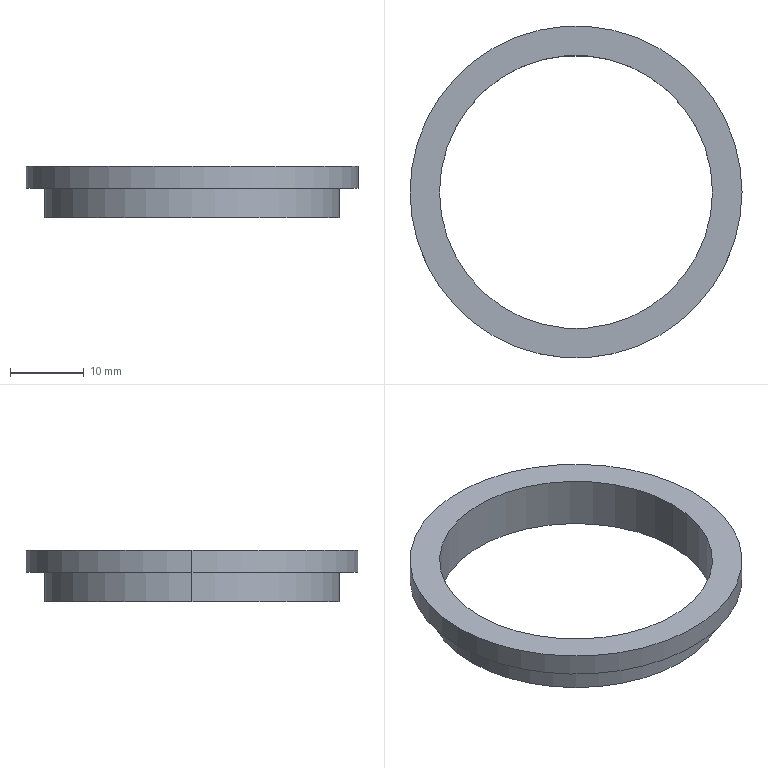Part | SolidWorks | features Extrusion 1, ICE 1 | 1 solid | 9 faces | box 45 x 45 x 7 mm | volume 2271 mm3 | cylinder 6 | plane 3 | commonest cylinder face diameters 37 x2 40 x2 45 x2
STEP:
#1=CARTESIAN_POINT('',(-20.,0.,-4.));
#2=VERTEX_POINT('',#1);
#3=CARTESIAN_POINT('',(20.,0.,-4.));
#4=VERTEX_POINT('',#3);
#5=CARTESIAN_POINT('',(0.,0.,-4.));
#6=DIRECTION('',(0.,0.,-1.));
#7=DIRECTION('',(-1.,0.,0.));
#8=AXIS2_PLACEMENT_3D('',#5,#6,#7);
#9=CIRCLE('',#8,20.);
#10=EDGE_CURVE('',#2,#4,#9,.T.);
#11=ORIENTED_EDGE('',*,*,#10,.F.);
#12=CARTESIAN_POINT('',(-20.,0.,0.));
#13=VERTEX_POINT('',#12);
#14=CARTESIAN_POINT('',(-20.,0.,-4.));
#15=DIRECTION('',(0.,0.,1.));
#16=VECTOR('',#15,1000.);
#17=LINE('',#14,#16);
#18=EDGE_CURVE('',#2,#13,#17,.T.);
#19=ORIENTED_EDGE('',*,*,#18,.T.);
#20=CARTESIAN_POINT('',(20.,0.,0.));
#21=VERTEX_POINT('',#20);
#22=CARTESIAN_POINT('',(0.,0.,0.));
#23=DIRECTION('',(0.,0.,-1.));
#24=DIRECTION('',(1.,0.,0.));
#25=AXIS2_PLACEMENT_3D('',#22,#23,#24);
#26=CIRCLE('',#25,20.);
#27=EDGE_CURVE('',#13,#21,#26,.T.);
#28=ORIENTED_EDGE('',*,*,#27,.T.);
#29=CARTESIAN_POINT('',(20.,0.,-4.));
#30=DIRECTION('',(0.,0.,1.));
#31=VECTOR('',#30,1000.);
#32=LINE('',#29,#31);
#33=EDGE_CURVE('',#4,#21,#32,.T.);
#34=ORIENTED_EDGE('',*,*,#33,.F.);
#35=EDGE_LOOP('',(#11,#19,#28,#34));
#36=FACE_OUTER_BOUND('',#35,.T.);
#37=CARTESIAN_POINT('',(0.,0.,-4.));
#38=DIRECTION('',(0.,0.,1.));
#39=DIRECTION('',(1.,0.,0.));
#40=AXIS2_PLACEMENT_3D('',#37,#38,#39);
#41=CYLINDRICAL_SURFACE('',#40,20.);
#42=ADVANCED_FACE('',(#36),#41,.T.);
#43=CARTESIAN_POINT('',(-18.5,0.,3.));
#44=VERTEX_POINT('',#43);
#45=CARTESIAN_POINT('',(18.5,0.,3.));
#46=VERTEX_POINT('',#45);
#47=CARTESIAN_POINT('',(0.,0.,3.));
#48=DIRECTION('',(0.,0.,1.));
#49=DIRECTION('',(1.,0.,0.));
#50=AXIS2_PLACEMENT_3D('',#47,#48,#49);
#51=CIRCLE('',#50,18.5);
#52=EDGE_CURVE('',#44,#46,#51,.T.);
#53=ORIENTED_EDGE('',*,*,#52,.T.);
#54=CARTESIAN_POINT('',(18.5,0.,-4.));
#55=VERTEX_POINT('',#54);
#56=CARTESIAN_POINT('',(18.5,0.,3.));
#57=DIRECTION('',(0.,0.,-1.));
#58=VECTOR('',#57,1000.);
#59=LINE('',#56,#58);
#60=EDGE_CURVE('',#46,#55,#59,.T.);
#61=ORIENTED_EDGE('',*,*,#60,.T.);
#62=CARTESIAN_POINT('',(-18.5,0.,-4.));
#63=VERTEX_POINT('',#62);
#64=CARTESIAN_POINT('',(0.,0.,-4.));
#65=DIRECTION('',(0.,0.,-1.));
#66=DIRECTION('',(-1.,0.,0.));
#67=AXIS2_PLACEMENT_3D('',#64,#65,#66);
#68=CIRCLE('',#67,18.5);
#69=EDGE_CURVE('',#55,#63,#68,.T.);
#70=ORIENTED_EDGE('',*,*,#69,.T.);
#71=CARTESIAN_POINT('',(-18.5,0.,3.));
#72=DIRECTION('',(0.,0.,-1.));
#73=VECTOR('',#72,1000.);
#74=LINE('',#71,#73);
#75=EDGE_CURVE('',#44,#63,#74,.T.);
#76=ORIENTED_EDGE('',*,*,#75,.F.);
#77=EDGE_LOOP('',(#53,#61,#70,#76));
#78=FACE_OUTER_BOUND('',#77,.T.);
#79=CARTESIAN_POINT('',(0.,0.,3.));
#80=DIRECTION('',(0.,0.,-1.));
#81=DIRECTION('',(-1.,0.,0.));
#82=AXIS2_PLACEMENT_3D('',#79,#80,#81);
#83=CYLINDRICAL_SURFACE('',#82,18.5);
#84=ADVANCED_FACE('',(#78),#83,.F.);
#85=CARTESIAN_POINT('',(22.5,0.,3.));
#86=VERTEX_POINT('',#85);
#87=CARTESIAN_POINT('',(-22.5,0.,3.));
#88=VERTEX_POINT('',#87);
#89=CARTESIAN_POINT('',(0.,0.,3.));
#90=DIRECTION('',(0.,0.,1.));
#91=DIRECTION('',(1.,0.,0.));
#92=AXIS2_PLACEMENT_3D('',#89,#90,#91);
#93=CIRCLE('',#92,22.5);
#94=EDGE_CURVE('',#86,#88,#93,.T.);
#95=ORIENTED_EDGE('',*,*,#94,.F.);
#96=CARTESIAN_POINT('',(22.5,0.,0.));
#97=VERTEX_POINT('',#96);
#98=CARTESIAN_POINT('',(22.5,0.,3.));
#99=DIRECTION('',(0.,0.,-1.));
#100=VECTOR('',#99,1000.);
#101=LINE('',#98,#100);
#102=EDGE_CURVE('',#86,#97,#101,.T.);
#103=ORIENTED_EDGE('',*,*,#102,.T.);
#104=CARTESIAN_POINT('',(-22.5,0.,0.));
#105=VERTEX_POINT('',#104);
#106=CARTESIAN_POINT('',(0.,0.,0.));
#107=DIRECTION('',(0.,0.,1.));
#108=DIRECTION('',(1.,0.,0.));
#109=AXIS2_PLACEMENT_3D('',#106,#107,#108);
#110=CIRCLE('',#109,22.5);
#111=EDGE_CURVE('',#97,#105,#110,.T.);
#112=ORIENTED_EDGE('',*,*,#111,.T.);
#113=CARTESIAN_POINT('',(-22.5,0.,3.));
#114=DIRECTION('',(0.,0.,-1.));
#115=VECTOR('',#114,1000.);
#116=LINE('',#113,#115);
#117=EDGE_CURVE('',#88,#105,#116,.T.);
#118=ORIENTED_EDGE('',*,*,#117,.F.);
#119=EDGE_LOOP('',(#95,#103,#112,#118));
#120=FACE_OUTER_BOUND('',#119,.T.);
#121=CARTESIAN_POINT('',(0.,0.,3.));
#122=DIRECTION('',(0.,0.,-1.));
#123=DIRECTION('',(-1.,0.,0.));
#124=AXIS2_PLACEMENT_3D('',#121,#122,#123);
#125=CYLINDRICAL_SURFACE('',#124,22.5);
#126=ADVANCED_FACE('',(#120),#125,.T.);
#127=CARTESIAN_POINT('',(0.,0.,0.));
#128=DIRECTION('',(0.,0.,1.));
#129=DIRECTION('',(1.,0.,0.));
#130=AXIS2_PLACEMENT_3D('',#127,#128,#129);
#131=CIRCLE('',#130,22.5);
#132=EDGE_CURVE('',#105,#97,#131,.T.);
#133=ORIENTED_EDGE('',*,*,#132,.F.);
#134=ORIENTED_EDGE('',*,*,#111,.F.);
#135=EDGE_LOOP('',(#133,#134));
#136=FACE_OUTER_BOUND('',#135,.T.);
#137=CARTESIAN_POINT('',(0.,0.,0.));
#138=DIRECTION('',(0.,0.,-1.));
#139=DIRECTION('',(1.,0.,0.));
#140=AXIS2_PLACEMENT_3D('',#137,#138,#139);
#141=CIRCLE('',#140,20.);
#142=EDGE_CURVE('',#21,#13,#141,.T.);
#143=ORIENTED_EDGE('',*,*,#142,.F.);
#144=ORIENTED_EDGE('',*,*,#27,.F.);
#145=EDGE_LOOP('',(#143,#144));
#146=FACE_BOUND('',#145,.T.);
#147=CARTESIAN_POINT('',(0.,0.,0.));
#148=DIRECTION('',(0.,0.,1.));
#149=DIRECTION('',(1.,0.,0.));
#150=AXIS2_PLACEMENT_3D('',#147,#148,#149);
#151=PLANE('',#150);
#152=ADVANCED_FACE('',(#136,#146),#151,.F.);
#153=CARTESIAN_POINT('',(0.,0.,3.));
#154=DIRECTION('',(0.,0.,1.));
#155=DIRECTION('',(1.,0.,0.));
#156=AXIS2_PLACEMENT_3D('',#153,#154,#155);
#157=CIRCLE('',#156,22.5);
#158=EDGE_CURVE('',#88,#86,#157,.T.);
#159=ORIENTED_EDGE('',*,*,#158,.T.);
#160=ORIENTED_EDGE('',*,*,#94,.T.);
#161=EDGE_LOOP('',(#159,#160));
#162=FACE_OUTER_BOUND('',#161,.T.);
#163=ORIENTED_EDGE('',*,*,#52,.F.);
#164=CARTESIAN_POINT('',(0.,0.,3.));
#165=DIRECTION('',(0.,0.,1.));
#166=DIRECTION('',(1.,0.,0.));
#167=AXIS2_PLACEMENT_3D('',#164,#165,#166);
#168=CIRCLE('',#167,18.5);
#169=EDGE_CURVE('',#46,#44,#168,.T.);
#170=ORIENTED_EDGE('',*,*,#169,.F.);
#171=EDGE_LOOP('',(#163,#170));
#172=FACE_BOUND('',#171,.T.);
#173=CARTESIAN_POINT('',(0.,0.,3.));
#174=DIRECTION('',(0.,0.,1.));
#175=DIRECTION('',(1.,0.,0.));
#176=AXIS2_PLACEMENT_3D('',#173,#174,#175);
#177=PLANE('',#176);
#178=ADVANCED_FACE('',(#162,#172),#177,.T.);
#179=ORIENTED_EDGE('',*,*,#102,.F.);
#180=ORIENTED_EDGE('',*,*,#158,.F.);
#181=ORIENTED_EDGE('',*,*,#117,.T.);
#182=ORIENTED_EDGE('',*,*,#132,.T.);
#183=EDGE_LOOP('',(#179,#180,#181,#182));
#184=FACE_OUTER_BOUND('',#183,.T.);
#185=CARTESIAN_POINT('',(0.,0.,3.));
#186=DIRECTION('',(0.,0.,-1.));
#187=DIRECTION('',(-1.,0.,0.));
#188=AXIS2_PLACEMENT_3D('',#185,#186,#187);
#189=CYLINDRICAL_SURFACE('',#188,22.5);
#190=ADVANCED_FACE('',(#184),#189,.T.);
#191=ORIENTED_EDGE('',*,*,#60,.F.);
#192=ORIENTED_EDGE('',*,*,#169,.T.);
#193=ORIENTED_EDGE('',*,*,#75,.T.);
#194=CARTESIAN_POINT('',(0.,0.,-4.));
#195=DIRECTION('',(0.,0.,-1.));
#196=DIRECTION('',(-1.,0.,0.));
#197=AXIS2_PLACEMENT_3D('',#194,#195,#196);
#198=CIRCLE('',#197,18.5);
#199=EDGE_CURVE('',#63,#55,#198,.T.);
#200=ORIENTED_EDGE('',*,*,#199,.T.);
#201=EDGE_LOOP('',(#191,#192,#193,#200));
#202=FACE_OUTER_BOUND('',#201,.T.);
#203=CARTESIAN_POINT('',(0.,0.,3.));
#204=DIRECTION('',(0.,0.,-1.));
#205=DIRECTION('',(-1.,0.,0.));
#206=AXIS2_PLACEMENT_3D('',#203,#204,#205);
#207=CYLINDRICAL_SURFACE('',#206,18.5);
#208=ADVANCED_FACE('',(#202),#207,.F.);
#209=CARTESIAN_POINT('',(0.,0.,-4.));
#210=DIRECTION('',(0.,0.,-1.));
#211=DIRECTION('',(-1.,0.,0.));
#212=AXIS2_PLACEMENT_3D('',#209,#210,#211);
#213=CIRCLE('',#212,20.);
#214=EDGE_CURVE('',#4,#2,#213,.T.);
#215=ORIENTED_EDGE('',*,*,#214,.T.);
#216=ORIENTED_EDGE('',*,*,#10,.T.);
#217=EDGE_LOOP('',(#215,#216));
#218=FACE_OUTER_BOUND('',#217,.T.);
#219=ORIENTED_EDGE('',*,*,#199,.F.);
#220=ORIENTED_EDGE('',*,*,#69,.F.);
#221=EDGE_LOOP('',(#219,#220));
#222=FACE_BOUND('',#221,.T.);
#223=CARTESIAN_POINT('',(0.,0.,-4.));
#224=DIRECTION('',(0.,0.,-1.));
#225=DIRECTION('',(-1.,0.,0.));
#226=AXIS2_PLACEMENT_3D('',#223,#224,#225);
#227=PLANE('',#226);
#228=ADVANCED_FACE('',(#218,#222),#227,.T.);
#229=ORIENTED_EDGE('',*,*,#18,.F.);
#230=ORIENTED_EDGE('',*,*,#214,.F.);
#231=ORIENTED_EDGE('',*,*,#33,.T.);
#232=ORIENTED_EDGE('',*,*,#142,.T.);
#233=EDGE_LOOP('',(#229,#230,#231,#232));
#234=FACE_OUTER_BOUND('',#233,.T.);
#235=CARTESIAN_POINT('',(0.,0.,-4.));
#236=DIRECTION('',(0.,0.,1.));
#237=DIRECTION('',(1.,0.,0.));
#238=AXIS2_PLACEMENT_3D('',#235,#236,#237);
#239=CYLINDRICAL_SURFACE('',#238,20.);
#240=ADVANCED_FACE('',(#234),#239,.T.);
#241=CLOSED_SHELL('',(#42,#84,#126,#152,#178,#190,#208,#228,#240));
#242=MANIFOLD_SOLID_BREP('',#241);
#243=CARTESIAN_POINT('',(0.,0.,0.));
#244=DIRECTION('',(0.,0.,1.));
#245=DIRECTION('',(1.,0.,0.));
#246=AXIS2_PLACEMENT_3D('',#243,#244,#245);
#247=(LENGTH_UNIT()NAMED_UNIT(*)SI_UNIT(.MILLI.,.METRE.));
#248=UNCERTAINTY_MEASURE_WITH_UNIT(LENGTH_MEASURE(0.00001),#247,'','');
#249=(NAMED_UNIT(*)PLANE_ANGLE_UNIT()SI_UNIT($,.RADIAN.));
#250=(NAMED_UNIT(*)SI_UNIT($,.STERADIAN.)SOLID_ANGLE_UNIT());
#251=(GEOMETRIC_REPRESENTATION_CONTEXT(3)GLOBAL_UNCERTAINTY_ASSIGNED_CONTEXT((#248))GLOBAL_UNIT_ASSIGNED_CONTEXT((#247,#249,#250))REPRESENTATION_CONTEXT('',''));
#252=ADVANCED_BREP_SHAPE_REPRESENTATION('',(#242,#246),#251);